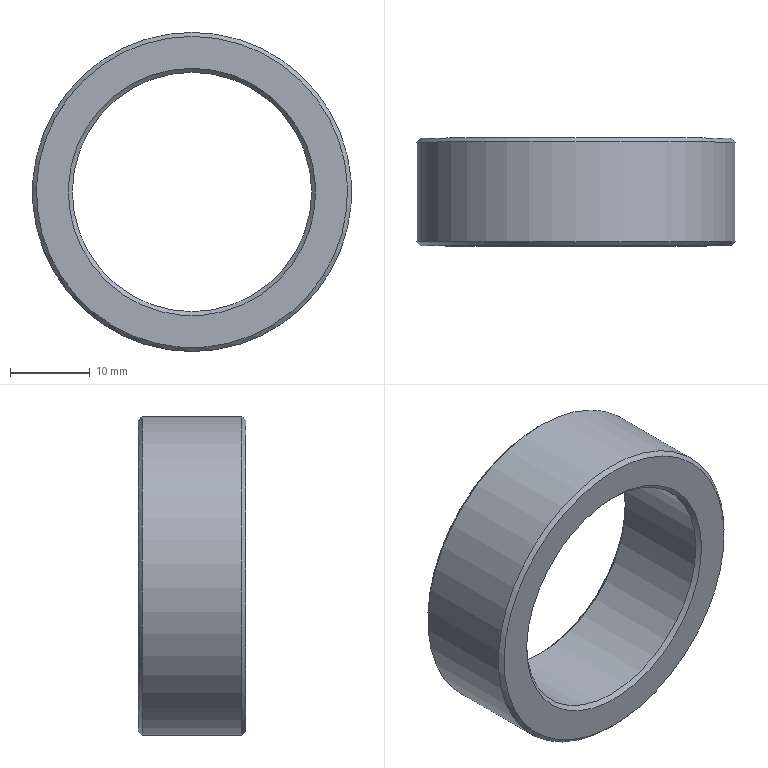Part | NX | features BREP 1, DATUM_CSYS 1 | 1 solid | 8 faces | box 40 x 13.5 x 40 mm | volume 7367 mm3 | cone 4 | cylinder 2 | plane 2 | commonest cylinder face diameters 30 x1 40 x1
STEP:
#1=CARTESIAN_POINT('',(160.,586.5,20.));
#2=VERTEX_POINT('',#1);
#3=CARTESIAN_POINT('',(160.,586.5,0.));
#4=DIRECTION('',(0.,1.,0.));
#5=DIRECTION('',(0.,0.,1.));
#6=AXIS2_PLACEMENT_3D('',#3,#4,#5);
#7=CIRCLE('',#6,20.);
#8=EDGE_CURVE('',#2,#2,#7,.T.);
#9=ORIENTED_EDGE('',*,*,#8,.T.);
#10=EDGE_LOOP('',(#9));
#11=FACE_BOUND('',#10,.T.);
#12=CARTESIAN_POINT('',(160.,599.,20.));
#13=VERTEX_POINT('',#12);
#14=CARTESIAN_POINT('',(160.,599.,0.));
#15=DIRECTION('',(0.,1.,0.));
#16=DIRECTION('',(0.,0.,1.));
#17=AXIS2_PLACEMENT_3D('',#14,#15,#16);
#18=CIRCLE('',#17,20.);
#19=EDGE_CURVE('',#13,#13,#18,.T.);
#20=ORIENTED_EDGE('',*,*,#19,.F.);
#21=EDGE_LOOP('',(#20));
#22=FACE_BOUND('',#21,.T.);
#23=CARTESIAN_POINT('',(160.,599.5,0.));
#24=DIRECTION('',(0.,1.,0.));
#25=DIRECTION('',(0.,0.,1.));
#26=AXIS2_PLACEMENT_3D('',#23,#24,#25);
#27=CYLINDRICAL_SURFACE('',#26,20.);
#28=ADVANCED_FACE('',(#11,#22),#27,.T.);
#29=CARTESIAN_POINT('',(160.,586.,19.5));
#30=VERTEX_POINT('',#29);
#31=CARTESIAN_POINT('',(160.,586.,0.));
#32=DIRECTION('',(0.,1.,0.));
#33=DIRECTION('',(0.,0.,1.));
#34=AXIS2_PLACEMENT_3D('',#31,#32,#33);
#35=CIRCLE('',#34,19.5);
#36=EDGE_CURVE('',#30,#30,#35,.T.);
#37=ORIENTED_EDGE('',*,*,#36,.T.);
#38=EDGE_LOOP('',(#37));
#39=FACE_BOUND('',#38,.T.);
#40=ORIENTED_EDGE('',*,*,#8,.F.);
#41=EDGE_LOOP('',(#40));
#42=FACE_BOUND('',#41,.T.);
#43=CARTESIAN_POINT('',(160.,586.5,0.));
#44=DIRECTION('',(0.,1.,0.));
#45=DIRECTION('',(0.,0.,1.));
#46=AXIS2_PLACEMENT_3D('',#43,#44,#45);
#47=CONICAL_SURFACE('',#46,20.,0.7854);
#48=ADVANCED_FACE('',(#39,#42),#47,.T.);
#49=CARTESIAN_POINT('',(160.,586.,15.5));
#50=VERTEX_POINT('',#49);
#51=CARTESIAN_POINT('',(160.,586.,0.));
#52=DIRECTION('',(0.,1.,0.));
#53=DIRECTION('',(0.,0.,1.));
#54=AXIS2_PLACEMENT_3D('',#51,#52,#53);
#55=CIRCLE('',#54,15.5);
#56=EDGE_CURVE('',#50,#50,#55,.T.);
#57=ORIENTED_EDGE('',*,*,#56,.T.);
#58=EDGE_LOOP('',(#57));
#59=FACE_BOUND('',#58,.T.);
#60=ORIENTED_EDGE('',*,*,#36,.F.);
#61=EDGE_LOOP('',(#60));
#62=FACE_BOUND('',#61,.T.);
#63=CARTESIAN_POINT('',(140.5,586.,0.));
#64=DIRECTION('',(0.,-1.,0.));
#65=DIRECTION('',(0.,0.,-1.));
#66=AXIS2_PLACEMENT_3D('',#63,#64,#65);
#67=PLANE('',#66);
#68=ADVANCED_FACE('',(#59,#62),#67,.T.);
#69=CARTESIAN_POINT('',(160.,586.5,15.));
#70=VERTEX_POINT('',#69);
#71=CARTESIAN_POINT('',(160.,586.5,0.));
#72=DIRECTION('',(0.,1.,0.));
#73=DIRECTION('',(0.,0.,1.));
#74=AXIS2_PLACEMENT_3D('',#71,#72,#73);
#75=CIRCLE('',#74,15.);
#76=EDGE_CURVE('',#70,#70,#75,.T.);
#77=ORIENTED_EDGE('',*,*,#76,.T.);
#78=EDGE_LOOP('',(#77));
#79=FACE_BOUND('',#78,.T.);
#80=ORIENTED_EDGE('',*,*,#56,.F.);
#81=EDGE_LOOP('',(#80));
#82=FACE_BOUND('',#81,.T.);
#83=CARTESIAN_POINT('',(160.,586.,0.));
#84=DIRECTION('',(0.,-1.,0.));
#85=DIRECTION('',(0.,0.,-1.));
#86=AXIS2_PLACEMENT_3D('',#83,#84,#85);
#87=CONICAL_SURFACE('',#86,15.5,0.7854);
#88=ADVANCED_FACE('',(#79,#82),#87,.F.);
#89=CARTESIAN_POINT('',(160.,599.,15.));
#90=VERTEX_POINT('',#89);
#91=CARTESIAN_POINT('',(160.,599.,0.));
#92=DIRECTION('',(0.,1.,0.));
#93=DIRECTION('',(0.,0.,1.));
#94=AXIS2_PLACEMENT_3D('',#91,#92,#93);
#95=CIRCLE('',#94,15.);
#96=EDGE_CURVE('',#90,#90,#95,.T.);
#97=ORIENTED_EDGE('',*,*,#96,.T.);
#98=EDGE_LOOP('',(#97));
#99=FACE_BOUND('',#98,.T.);
#100=ORIENTED_EDGE('',*,*,#76,.F.);
#101=EDGE_LOOP('',(#100));
#102=FACE_BOUND('',#101,.T.);
#103=CARTESIAN_POINT('',(160.,599.5,0.));
#104=DIRECTION('',(0.,1.,0.));
#105=DIRECTION('',(0.,0.,1.));
#106=AXIS2_PLACEMENT_3D('',#103,#104,#105);
#107=CYLINDRICAL_SURFACE('',#106,15.);
#108=ADVANCED_FACE('',(#99,#102),#107,.F.);
#109=CARTESIAN_POINT('',(160.,599.5,15.5));
#110=VERTEX_POINT('',#109);
#111=CARTESIAN_POINT('',(160.,599.5,0.));
#112=DIRECTION('',(0.,1.,0.));
#113=DIRECTION('',(0.,0.,1.));
#114=AXIS2_PLACEMENT_3D('',#111,#112,#113);
#115=CIRCLE('',#114,15.5);
#116=EDGE_CURVE('',#110,#110,#115,.T.);
#117=ORIENTED_EDGE('',*,*,#116,.T.);
#118=EDGE_LOOP('',(#117));
#119=FACE_BOUND('',#118,.T.);
#120=ORIENTED_EDGE('',*,*,#96,.F.);
#121=EDGE_LOOP('',(#120));
#122=FACE_BOUND('',#121,.T.);
#123=CARTESIAN_POINT('',(160.,599.,0.));
#124=DIRECTION('',(0.,1.,0.));
#125=DIRECTION('',(0.,0.,1.));
#126=AXIS2_PLACEMENT_3D('',#123,#124,#125);
#127=CONICAL_SURFACE('',#126,15.,0.7854);
#128=ADVANCED_FACE('',(#119,#122),#127,.F.);
#129=CARTESIAN_POINT('',(160.,599.5,19.5));
#130=VERTEX_POINT('',#129);
#131=CARTESIAN_POINT('',(160.,599.5,0.));
#132=DIRECTION('',(0.,1.,0.));
#133=DIRECTION('',(0.,0.,1.));
#134=AXIS2_PLACEMENT_3D('',#131,#132,#133);
#135=CIRCLE('',#134,19.5);
#136=EDGE_CURVE('',#130,#130,#135,.T.);
#137=ORIENTED_EDGE('',*,*,#136,.T.);
#138=EDGE_LOOP('',(#137));
#139=FACE_BOUND('',#138,.T.);
#140=ORIENTED_EDGE('',*,*,#116,.F.);
#141=EDGE_LOOP('',(#140));
#142=FACE_BOUND('',#141,.T.);
#143=CARTESIAN_POINT('',(144.5,599.5,0.));
#144=DIRECTION('',(0.,1.,0.));
#145=DIRECTION('',(0.,0.,1.));
#146=AXIS2_PLACEMENT_3D('',#143,#144,#145);
#147=PLANE('',#146);
#148=ADVANCED_FACE('',(#139,#142),#147,.T.);
#149=ORIENTED_EDGE('',*,*,#19,.T.);
#150=EDGE_LOOP('',(#149));
#151=FACE_BOUND('',#150,.T.);
#152=ORIENTED_EDGE('',*,*,#136,.F.);
#153=EDGE_LOOP('',(#152));
#154=FACE_BOUND('',#153,.T.);
#155=CARTESIAN_POINT('',(160.,599.5,0.));
#156=DIRECTION('',(0.,-1.,0.));
#157=DIRECTION('',(0.,0.,-1.));
#158=AXIS2_PLACEMENT_3D('',#155,#156,#157);
#159=CONICAL_SURFACE('',#158,19.5,0.7854);
#160=ADVANCED_FACE('',(#151,#154),#159,.T.);
#161=CLOSED_SHELL('',(#28,#48,#68,#88,#108,#128,#148,#160));
#162=MANIFOLD_SOLID_BREP('',#161);
#163=(LENGTH_UNIT()NAMED_UNIT(*)SI_UNIT(.MILLI.,.METRE.));
#164=UNCERTAINTY_MEASURE_WITH_UNIT(LENGTH_MEASURE(0.00001),#163,'','');
#165=(NAMED_UNIT(*)PLANE_ANGLE_UNIT()SI_UNIT($,.RADIAN.));
#166=(NAMED_UNIT(*)SI_UNIT($,.STERADIAN.)SOLID_ANGLE_UNIT());
#167=(GEOMETRIC_REPRESENTATION_CONTEXT(3)GLOBAL_UNCERTAINTY_ASSIGNED_CONTEXT((#164))GLOBAL_UNIT_ASSIGNED_CONTEXT((#163,#165,#166))REPRESENTATION_CONTEXT('',''));
#168=ADVANCED_BREP_SHAPE_REPRESENTATION('',(#162),#167);